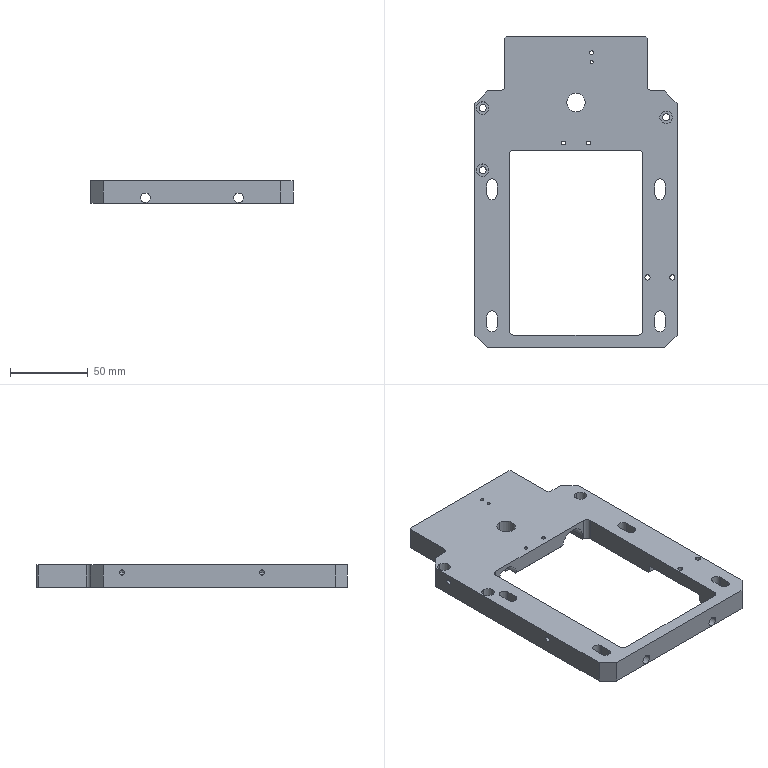NC program | NX | posted with a generic post | part box 130 x 200 x 14.5 mm
Lines 9720 to 10693 of 25347:
(ZLEVEL_PROFILE_COPY_COPY , TOOL : D4)
N19366 T17 M6
N19368 G54
N19370 G17 G0 G90 X24.194 Y-32.123 B0. C0. S5500 M3
N19372 G43 Z30. H17
N19374 Z-10.4
N19376 G94 G1 X24.463 Y-32.638 F1000.
N19378 G3 X24.8 Y-32.852 R0.4
N19380 G1 X27. Y-32.945 F1650.
N19382 X100.
N19384 X102.199 Y-32.852
N19386 Y-32.784 Z-10.45
N19388 Y-32.693 Z-10.5
N19390 X100.326 Y-32.74
N19392 X100. Y-32.792
N19394 X27.
N19396 X26.674 Y-32.74
N19398 X24.8 Y-32.693
N19400 Y-32.624 Z-10.55
N19402 Y-32.534 Z-10.6
N19404 X26.674 Y-32.58
N19406 X27. Y-32.631
N19408 X100.
N19410 X100.326 Y-32.58
N19412 X102.199 Y-32.534
N19414 Y-32.454 Z-10.65
N19416 Y-32.365 Z-10.7
N19418 X99.839 Y-32.463
N19420 X27.
N19422 X26.674 Y-32.416
N19424 X24.8 Y-32.365
N19426 Y-32.274 Z-10.75
N19428 Y-32.186 Z-10.8
N19430 X26.674 Y-32.236
N19432 X27. Y-32.286
N19434 X100.
N19436 X100.326 Y-32.236
N19438 X102.199 Y-32.186
N19440 Y-32.095 Z-10.85
N19442 Y-32.006 Z-10.9
N19444 X100.326 Y-32.056
N19446 X100. Y-32.099
N19448 X27.
N19450 X26.674 Y-32.056
N19452 X24.8 Y-32.006
N19454 Y-31.893 Z-10.95
N19456 Y-31.793 Z-11.
N19458 X27. Y-31.9
N19460 X100.
N19462 X102.199 Y-31.793
N19464 Y-31.68 Z-11.05
N19466 Y-31.567 Z-11.1
N19468 X100. Y-31.688
N19470 X27.
N19472 X24.8 Y-31.567
N19474 Y-31.453 Z-11.15
N19476 Y-31.326 Z-11.2
N19478 X26.674 Y-31.392
N19480 X27. Y-31.46
N19482 X100.
N19484 X100.326 Y-31.392
N19486 X102.199 Y-31.326
N19488 Y-31.207 Z-11.25
N19490 Y-31.071 Z-11.3
N19492 X100.326 Y-31.136
N19494 X100. Y-31.212
N19496 X27.
N19498 X26.674 Y-31.136
N19500 X24.8 Y-31.071
N19502 Y-30.937 Z-11.35
N19504 Y-30.789 Z-11.4
N19506 X26.674 Y-30.863
N19508 X27. Y-30.941
N19510 X100.
N19512 X100.326 Y-30.863
N19514 X102.199 Y-30.789
N19516 Y-30.638 Z-11.45
N19518 Y-30.49 Z-11.5
N19520 X100.326 Y-30.564
N19522 X100. Y-30.638
N19524 X27.
N19526 X26.674 Y-30.564
N19528 X24.8 Y-30.49
N19530 Y-30.304 Z-11.55
N19532 Y-30.088 Z-11.6
N19534 G2 X27. Y-30.291 R5.952
N19536 G1 X100.
N19538 G2 X102.2 Y-30.088 R6.111
N19540 G3 X102.563 Y-29.92 R0.4
N19542 G1 X104.065 Y-30.
N19544 G0 Z30.
N19546 X102.806 Y-27.877
N19548 Z-10.4
N19550 G1 X102.537 Y-27.362 F1000.
N19552 G3 X102.199 Y-27.148 R0.4
N19554 G1 X100. Y-27.055 F1650.
N19556 X27.
N19558 X24.8 Y-27.148
N19560 Y-27.216 Z-10.45
N19562 Y-27.307 Z-10.5
N19564 X26.674 Y-27.26
N19566 X27. Y-27.208
N19568 X100.
N19570 X100.326 Y-27.26
N19572 X102.199 Y-27.307
N19574 Y-27.376 Z-10.55
N19576 Y-27.466 Z-10.6
N19578 X100.326 Y-27.42
N19580 X100. Y-27.369
N19582 X27.
N19584 X26.674 Y-27.42
N19586 X24.8 Y-27.466
N19588 Y-27.546 Z-10.65
N19590 Y-27.635 Z-10.7
N19592 X26.674 Y-27.584
N19594 X27. Y-27.537
N19596 X99.839
N19598 X102.199 Y-27.635
N19600 Y-27.726 Z-10.75
N19602 Y-27.814 Z-10.8
N19604 X100.326 Y-27.764
N19606 X100. Y-27.714
N19608 X27.
N19610 X26.674 Y-27.764
N19612 X24.8 Y-27.814
N19614 Y-27.905 Z-10.85
N19616 Y-27.994 Z-10.9
N19618 X26.674 Y-27.944
N19620 X27. Y-27.901
N19622 X100.
N19624 X100.326 Y-27.944
N19626 X102.199 Y-27.994
N19628 Y-28.107 Z-10.95
N19630 Y-28.207 Z-11.
N19632 X100. Y-28.1
N19634 X27.
N19636 X24.8 Y-28.207
N19638 Y-28.32 Z-11.05
N19640 Y-28.433 Z-11.1
N19642 X27. Y-28.312
N19644 X100.
N19646 X102.199 Y-28.433
N19648 Y-28.547 Z-11.15
N19650 Y-28.674 Z-11.2
N19652 X100.326 Y-28.608
N19654 X100. Y-28.54
N19656 X27.
N19658 X26.674 Y-28.608
N19660 X24.8 Y-28.674
N19662 Y-28.793 Z-11.25
N19664 Y-28.929 Z-11.3
N19666 X26.674 Y-28.864
N19668 X27. Y-28.788
N19670 X100.
N19672 X100.326 Y-28.864
N19674 X102.199 Y-28.929
N19676 Y-29.063 Z-11.35
N19678 Y-29.211 Z-11.4
N19680 X100.326 Y-29.137
N19682 X100. Y-29.059
N19684 X27.
N19686 X26.674 Y-29.137
N19688 X24.8 Y-29.211
N19690 Y-29.362 Z-11.45
N19692 Y-29.51 Z-11.5
N19694 X26.674 Y-29.436
N19696 X27. Y-29.362
N19698 X100.
N19700 X100.326 Y-29.436
N19702 X102.199 Y-29.51
N19704 X102.2 Y-29.698 Z-11.55
N19706 Y-29.912 Z-11.6
N19708 G2 X100. Y-29.709 R5.952
N19710 G1 X27.
N19712 G2 X24.8 Y-29.912 R6.115
N19714 G3 X24.437 Y-30.08 R0.4
N19716 G1 X22.935 Y-30.
N19718 G0 Z30.
N19720 X102.825 Y32.137
N19722 Z-10.4
N19724 G1 X102.542 Y32.651 F1000.
N19726 G3 X102.199 Y32.857 R0.4
N19728 G1 X100.42 Y32.892 F1650.
N19730 X100. Y32.945
N19732 X27.
N19734 X24.8 Y32.854
N19736 Y32.785 Z-10.45
N19738 Y32.705 Z-10.5
N19740 X26.68 Y32.748
N19742 X27. Y32.792
N19744 X100.
N19746 X100.42 Y32.742
N19748 X102.199 Y32.708
N19750 Y32.623 Z-10.55
N19752 Y32.548 Z-10.6
N19754 X100. Y32.631
N19756 X27.
N19758 X24.8 Y32.545
N19760 Y32.454 Z-10.65
N19762 Y32.365 Z-10.7
N19764 X26.68 Y32.417
N19766 X27. Y32.463
N19768 X100.
N19770 X100.42 Y32.409
N19772 X102.199 Y32.369
N19774 Y32.274 Z-10.75
N19776 Y32.189 Z-10.8
N19778 X100.42 Y32.23
N19780 X100. Y32.286
N19782 X27.
N19784 X26.68 Y32.237
N19786 X24.8 Y32.186
N19788 Y32.094 Z-10.85
N19790 Y31.988 Z-10.9
N19792 X26.68 Y32.047
N19794 X27. Y32.099
N19796 X100.
N19798 X100.42 Y32.038
N19800 X102.199 Y31.992
N19802 Y31.894 Z-10.95
N19804 Y31.785 Z-11.
N19806 X100.42 Y31.83
N19808 X100. Y31.9
N19810 X27.
N19812 X26.68 Y31.838
N19814 X24.8 Y31.781
N19816 Y31.68 Z-11.05
N19818 Y31.566 Z-11.1
N19820 X26.832 Y31.642
N19822 X27. Y31.688
N19824 X100.
N19826 X100.168 Y31.642
N19828 X102.199 Y31.57
N19830 Y31.453 Z-11.15
N19832 Y31.338 Z-11.2
N19834 X101.885 Y31.334
N19836 X100. Y31.46
N19838 X27.
N19840 X26.68 Y31.395
N19842 X24.8 Y31.335
N19844 Y31.207 Z-11.25
N19846 Y31.087 Z-11.3
N19848 X26.68 Y31.161
N19850 X27. Y31.212
N19852 X100.
N19854 X101.885 Y31.086
N19856 X102.199 Y31.091
N19858 Y30.937 Z-11.35
N19860 Y30.792 Z-11.4
N19862 X100.42 Y30.852
N19864 X100. Y30.941
N19866 X27.
N19868 X26.68 Y30.864
N19870 X24.8 Y30.789
N19872 Y30.637 Z-11.45
N19874 Y30.459 Z-11.5
N19876 X26.68 Y30.545
N19878 X27. Y30.638
N19880 X100.
N19882 X100.42 Y30.531
N19884 X102.199 Y30.463
N19886 X102.201 Y30.304 Z-11.55
N19888 X102.204 Y30.092 Z-11.6
N19890 G2 X100. Y30.291 R6.23
N19892 G1 X27.
N19894 G2 X24.803 Y30.092 R6.337
N19896 G3 X24.441 Y29.921 R0.4
N19898 G1 X22.932 Y29.999
N19900 G0 Z30.
N19902 X24.191 Y27.869
N19904 Z-10.4
N19906 G1 X24.462 Y27.354 F1000.
N19908 G3 X24.8 Y27.141 R0.4
N19910 G1 X27. Y27.055 F1650.
N19912 X100.
N19914 X100.42 Y27.102
N19916 X102.199 Y27.137
N19918 Y27.215 Z-10.45
N19920 Y27.283 Z-10.5
N19922 X100.42 Y27.248
N19924 X100. Y27.208
N19926 X27.
N19928 X24.8 Y27.287
N19930 Y27.377 Z-10.55
N19932 Y27.462 Z-10.6
N19934 X27. Y27.369
N19936 X100.
N19938 X100.42 Y27.416
N19940 X102.199 Y27.458
N19942 Y27.546 Z-10.65
N19944 Y27.634 Z-10.7
N19946 X100.42 Y27.593
N19948 X100. Y27.537
N19950 X27.
N19952 X26.68 Y27.586
N19954 X24.8 Y27.638
N19956 Y27.726 Z-10.75
N19958 Y27.818 Z-10.8
N19960 X26.68 Y27.763
N19962 X27. Y27.714
N19964 X100.
N19966 X100.42 Y27.77
N19968 X102.199 Y27.814
N19970 Y27.906 Z-10.85
N19972 Y28.012 Z-10.9
N19974 X100.42 Y27.968
N19976 X100. Y27.901
N19978 X27.
N19980 X26.68 Y27.96
N19982 X24.8 Y28.015
N19984 Y28.105 Z-10.95
N19986 Y28.213 Z-11.
N19988 X26.68 Y28.159
N19990 X27. Y28.1
N19992 X100.
N19994 X100.42 Y28.167
N19996 X102.199 Y28.209
N19998 Y28.32 Z-11.05
N20000 Y28.429 Z-11.1
N20002 X101.885 Y28.433
N20004 X100. Y28.312
N20006 X27.
N20008 X24.8 Y28.432
N20010 Y28.547 Z-11.15
N20012 Y28.659 Z-11.2
N20014 X27. Y28.54
N20016 X100.
N20018 X101.885 Y28.66
N20020 X102.199 Y28.655
N20022 Y28.794 Z-11.25
N20024 Y28.92 Z-11.3
N20026 X100.42 Y28.859
N20028 X100. Y28.788
N20030 X27.
N20032 X26.68 Y28.848
N20034 X24.8 Y28.924
N20036 Y29.063 Z-11.35
N20038 Y29.212 Z-11.4
N20040 X26.68 Y29.139
N20042 X27. Y29.059
N20044 X100.
N20046 X100.42 Y29.15
N20048 X102.199 Y29.208
N20050 Y29.362 Z-11.45
N20052 Y29.532 Z-11.5
N20054 X100.42 Y29.47
N20056 X100. Y29.362
N20058 X27.
N20060 X26.68 Y29.457
N20062 X24.8 Y29.535
N20064 X24.801 Y29.696 Z-11.55
N20066 X24.803 Y29.908 Z-11.6
N20068 G2 X27. Y29.709 R6.152
N20070 G1 X100.
N20072 G2 X102.207 Y29.908 R6.355
N20074 G3 X102.569 Y30.078 R0.4
N20076 G1 X104.062 Y29.991
N20078 G0 Z30.
(ZLEVEL_PROFILE_COPY_COPY_COPY , TOOL : D4)
N20080 X-86.41 Y40.2
N20082 Z-0.1
N20084 G1 X-86.757 Y40.8 F1000.
N20086 G3 X-87.103 Y41. R0.4
N20088 G1 X-89. F1650.
N20090 G3 X-90. Y40. R1.
N20092 G1 Y38.103
N20094 G3 X-89.8 Y37.757 R0.4
N20096 G1 X-89.2 Y37.41
N20098 G0 X-86.41 Y40.2 Z-0.2
N20100 G1 X-86.757 Y40.8 F1000.
N20102 G3 X-87.103 Y41. R0.4
N20104 G1 X-89. F1650.
N20106 G3 X-90. Y40. R1.
N20108 G1 Y38.103
N20110 G3 X-89.8 Y37.757 R0.4
N20112 G1 X-89.2 Y37.41
N20114 G0 X-86.41 Y40.2 Z-0.3
N20116 G1 X-86.757 Y40.8 F1000.
N20118 G3 X-87.103 Y41. R0.4
N20120 G1 X-89. F1650.
N20122 G3 X-90. Y40. R1.
N20124 G1 Y38.103
N20126 G3 X-89.8 Y37.757 R0.4
N20128 G1 X-89.2 Y37.41
N20130 G0 X-86.41 Y40.2 Z-0.4
N20132 G1 X-86.757 Y40.8 F1000.
N20134 G3 X-87.103 Y41. R0.4
N20136 G1 X-89. F1650.
N20138 G3 X-90. Y40. R1.
N20140 G1 Y38.103
N20142 G3 X-89.8 Y37.757 R0.4
N20144 G1 X-89.2 Y37.41
N20146 G0 X-86.41 Y40.2 Z-0.5
N20148 G1 X-86.757 Y40.8 F1000.
N20150 G3 X-87.103 Y41. R0.4
N20152 G1 X-89. F1650.
N20154 G3 X-90. Y40. R1.
N20156 G1 Y38.103
N20158 G3 X-89.8 Y37.757 R0.4
N20160 G1 X-89.2 Y37.41
N20162 G0 X-86.41 Y40.2 Z-0.6
N20164 G1 X-86.757 Y40.8 F1000.
N20166 G3 X-87.103 Y41. R0.4
N20168 G1 X-89. F1650.
N20170 G3 X-90. Y40. R1.
N20172 G1 Y38.103
N20174 G3 X-89.8 Y37.757 R0.4
N20176 G1 X-89.2 Y37.41
N20178 G0 X-86.41 Y40.2 Z-0.7
N20180 G1 X-86.757 Y40.8 F1000.
N20182 G3 X-87.103 Y41. R0.4
N20184 G1 X-89. F1650.
N20186 G3 X-90. Y40. R1.
N20188 G1 Y38.103
N20190 G3 X-89.8 Y37.757 R0.4
N20192 G1 X-89.2 Y37.41
N20194 G0 X-86.41 Y40.2 Z-0.8
N20196 G1 X-86.757 Y40.8 F1000.
N20198 G3 X-87.103 Y41. R0.4
N20200 G1 X-89. F1650.
N20202 G3 X-90. Y40. R1.
N20204 G1 Y38.103
N20206 G3 X-89.8 Y37.757 R0.4
N20208 G1 X-89.2 Y37.41
N20210 G0 X-86.41 Y40.2 Z-0.9
N20212 G1 X-86.757 Y40.8 F1000.
N20214 G3 X-87.103 Y41. R0.4
N20216 G1 X-89. F1650.
N20218 G3 X-90. Y40. R1.
N20220 G1 Y38.103
N20222 G3 X-89.8 Y37.757 R0.4
N20224 G1 X-89.2 Y37.41
N20226 G0 X-86.41 Y40.2 Z-1.
N20228 G1 X-86.757 Y40.8 F1000.
N20230 G3 X-87.103 Y41. R0.4
N20232 G1 X-89. F1650.
N20234 G3 X-90. Y40. R1.
N20236 G1 Y38.103
N20238 G3 X-89.8 Y37.757 R0.4
N20240 G1 X-89.2 Y37.41
N20242 G0 X-86.41 Y40.2 Z-1.1
N20244 G1 X-86.757 Y40.8 F1000.
N20246 G3 X-87.103 Y41. R0.4
N20248 G1 X-89. F1650.
N20250 G3 X-90. Y40. R1.
N20252 G1 Y38.103
N20254 G3 X-89.8 Y37.757 R0.4
N20256 G1 X-89.2 Y37.41
N20258 G0 X-86.41 Y40.2 Z-1.2
N20260 G1 X-86.757 Y40.8 F1000.
N20262 G3 X-87.103 Y41. R0.4
N20264 G1 X-89. F1650.
N20266 G3 X-90. Y40. R1.
N20268 G1 Y38.103
N20270 G3 X-89.8 Y37.757 R0.4
N20272 G1 X-89.2 Y37.41
N20274 G0 X-86.41 Y40.2 Z-1.3
N20276 G1 X-86.757 Y40.8 F1000.
N20278 G3 X-87.103 Y41. R0.4
N20280 G1 X-89. F1650.
N20282 G3 X-90. Y40. R1.
N20284 G1 Y38.103
N20286 G3 X-89.8 Y37.757 R0.4
N20288 G1 X-89.2 Y37.41
N20290 G0 X-86.41 Y40.2 Z-1.4
N20292 G1 X-86.757 Y40.8 F1000.
N20294 G3 X-87.103 Y41. R0.4
N20296 G1 X-89. F1650.
N20298 G3 X-90. Y40. R1.
N20300 G1 Y38.103
N20302 G3 X-89.8 Y37.757 R0.4
N20304 G1 X-89.2 Y37.41
N20306 G0 X-86.41 Y40.2 Z-1.5
N20308 G1 X-86.757 Y40.8 F1000.
N20310 G3 X-87.103 Y41. R0.4
N20312 G1 X-89. F1650.
N20314 G3 X-90. Y40. R1.
N20316 G1 Y38.103
N20318 G3 X-89.8 Y37.757 R0.4
N20320 G1 X-89.2 Y37.41
N20322 G0 X-86.41 Y40.2 Z-1.6
N20324 G1 X-86.757 Y40.8 F1000.
N20326 G3 X-87.103 Y41. R0.4
N20328 G1 X-89. F1650.
N20330 G3 X-90. Y40. R1.
N20332 G1 Y38.103
N20334 G3 X-89.8 Y37.757 R0.4
N20336 G1 X-89.2 Y37.41
N20338 G0 X-86.41 Y40.2 Z-1.7
N20340 G1 X-86.757 Y40.8 F1000.
N20342 G3 X-87.103 Y41. R0.4
N20344 G1 X-89. F1650.
N20346 G3 X-90. Y40. R1.
N20348 G1 Y38.103
N20350 G3 X-89.8 Y37.757 R0.4
N20352 G1 X-89.2 Y37.41
N20354 G0 X-86.41 Y40.2 Z-1.8
N20356 G1 X-86.757 Y40.8 F1000.
N20358 G3 X-87.103 Y41. R0.4
N20360 G1 X-89. F1650.
N20362 G3 X-90. Y40. R1.
N20364 G1 Y38.103
N20366 G3 X-89.8 Y37.757 R0.4
N20368 G1 X-89.2 Y37.41
N20370 G0 X-86.41 Y40.2 Z-1.9
N20372 G1 X-86.757 Y40.8 F1000.
N20374 G3 X-87.103 Y41. R0.4
N20376 G1 X-89. F1650.
N20378 G3 X-90. Y40. R1.
N20380 G1 Y38.103
N20382 G3 X-89.8 Y37.757 R0.4
N20384 G1 X-89.2 Y37.41
N20386 G0 X-86.41 Y40.2 Z-2.
N20388 G1 X-86.757 Y40.8 F1000.
N20390 G3 X-87.103 Y41. R0.4
N20392 G1 X-89. F1650.
N20394 G3 X-90. Y40. R1.
N20396 G1 Y38.103
N20398 G3 X-89.8 Y37.757 R0.4
N20400 G1 X-89.2 Y37.41
N20402 G0 X-86.41 Y40.2 Z-2.1
N20404 G1 X-86.757 Y40.8 F1000.
N20406 G3 X-87.103 Y41. R0.4
N20408 G1 X-89. F1650.
N20410 G3 X-90. Y40. R1.
N20412 G1 Y38.103
N20414 G3 X-89.8 Y37.757 R0.4
N20416 G1 X-89.2 Y37.41
N20418 G0 X-86.41 Y40.2 Z-2.2
N20420 G1 X-86.757 Y40.8 F1000.
N20422 G3 X-87.103 Y41. R0.4
N20424 G1 X-89. F1650.
N20426 G3 X-90. Y40. R1.
N20428 G1 Y38.103
N20430 G3 X-89.8 Y37.757 R0.4
N20432 G1 X-89.2 Y37.41
N20434 G0 X-86.41 Y40.2 Z-2.3
N20436 G1 X-86.757 Y40.8 F1000.
N20438 G3 X-87.103 Y41. R0.4
N20440 G1 X-89. F1650.
N20442 G3 X-90. Y40. R1.
N20444 G1 Y38.103
N20446 G3 X-89.8 Y37.757 R0.4
N20448 G1 X-89.2 Y37.41
N20450 G0 X-86.41 Y40.2 Z-2.4
N20452 G1 X-86.757 Y40.8 F1000.
N20454 G3 X-87.103 Y41. R0.4
N20456 G1 X-89. F1650.
N20458 G3 X-90. Y40. R1.
N20460 G1 Y38.103
N20462 G3 X-89.8 Y37.757 R0.4
N20464 G1 X-89.2 Y37.41
N20466 G0 X-86.41 Y40.2 Z-2.5
N20468 G1 X-86.757 Y40.8 F1000.
N20470 G3 X-87.103 Y41. R0.4
N20472 G1 X-89. F1650.
N20474 G3 X-90. Y40. R1.
N20476 G1 Y38.103
N20478 G3 X-89.8 Y37.757 R0.4
N20480 G1 X-89.2 Y37.41
N20482 G0 X-86.41 Y40.2 Z-2.6
N20484 G1 X-86.757 Y40.8 F1000.
N20486 G3 X-87.103 Y41. R0.4
N20488 G1 X-89. F1650.
N20490 G3 X-90. Y40. R1.
N20492 G1 Y38.103
N20494 G3 X-89.8 Y37.757 R0.4
N20496 G1 X-89.2 Y37.41
N20498 G0 X-86.41 Y40.2 Z-2.7
N20500 G1 X-86.757 Y40.8 F1000.
N20502 G3 X-87.103 Y41. R0.4
N20504 G1 X-89. F1650.
N20506 G3 X-90. Y40. R1.
N20508 G1 Y38.103
N20510 G3 X-89.8 Y37.757 R0.4
N20512 G1 X-89.2 Y37.41
N20514 G0 X-86.41 Y40.2 Z-2.8
N20516 G1 X-86.757 Y40.8 F1000.
N20518 G3 X-87.103 Y41. R0.4
N20520 G1 X-89. F1650.
N20522 G3 X-90. Y40. R1.
N20524 G1 Y38.103
N20526 G3 X-89.8 Y37.757 R0.4
N20528 G1 X-89.2 Y37.41
N20530 G0 X-86.41 Y40.2 Z-2.9
N20532 G1 X-86.757 Y40.8 F1000.
N20534 G3 X-87.103 Y41. R0.4
N20536 G1 X-89. F1650.
N20538 G3 X-90. Y40. R1.
N20540 G1 Y38.103
N20542 G3 X-89.8 Y37.757 R0.4
N20544 G1 X-89.2 Y37.41
N20546 G0 X-86.41 Y40.2 Z-3.
N20548 G1 X-86.757 Y40.8 F1000.
N20550 G3 X-87.103 Y41. R0.4
N20552 G1 X-89. F1650.
N20554 G3 X-90. Y40. R1.
N20556 G1 Y38.103
N20558 G3 X-89.8 Y37.757 R0.4
N20560 G1 X-89.2 Y37.41
N20562 G0 X-86.41 Y40.2 Z-3.1
N20564 G1 X-86.757 Y40.8 F1000.
N20566 G3 X-87.103 Y41. R0.4
N20568 G1 X-89. F1650.
N20570 G3 X-90. Y40. R1.
N20572 G1 Y38.103
N20574 G3 X-89.8 Y37.757 R0.4
N20576 G1 X-89.2 Y37.41
N20578 G0 X-86.41 Y40.2 Z-3.2
N20580 G1 X-86.757 Y40.8 F1000.
N20582 G3 X-87.103 Y41. R0.4
N20584 G1 X-89. F1650.
N20586 G3 X-90. Y40. R1.
N20588 G1 Y38.103
N20590 G3 X-89.8 Y37.757 R0.4
N20592 G1 X-89.2 Y37.41
N20594 G0 X-86.41 Y40.2 Z-3.3
N20596 G1 X-86.757 Y40.8 F1000.
N20598 G3 X-87.103 Y41. R0.4
N20600 G1 X-89. F1650.
N20602 G3 X-90. Y40. R1.
N20604 G1 Y38.103
N20606 G3 X-89.8 Y37.757 R0.4
N20608 G1 X-89.2 Y37.41
N20610 G0 X-86.41 Y40.2 Z-3.4
N20612 G1 X-86.757 Y40.8 F1000.
N20614 G3 X-87.103 Y41. R0.4
N20616 G1 X-89. F1650.
N20618 G3 X-90. Y40. R1.
N20620 G1 Y38.103
N20622 G3 X-89.8 Y37.757 R0.4
N20624 G1 X-89.2 Y37.41
N20626 G0 X-86.41 Y40.2 Z-3.5
N20628 G1 X-86.757 Y40.8 F1000.
N20630 G3 X-87.103 Y41. R0.4
N20632 G1 X-89. F1650.
N20634 G3 X-90. Y40. R1.
N20636 G1 Y38.103
N20638 G3 X-89.8 Y37.757 R0.4
N20640 G1 X-89.2 Y37.41
N20642 G0 X-86.41 Y40.2 Z-3.6
N20644 G1 X-86.757 Y40.8 F1000.
N20646 G3 X-87.103 Y41. R0.4
N20648 G1 X-89. F1650.
N20650 G3 X-90. Y40. R1.
N20652 G1 Y38.103
N20654 G3 X-89.8 Y37.757 R0.4
N20656 G1 X-89.2 Y37.41
N20658 G0 X-86.41 Y40.2 Z-3.7
N20660 G1 X-86.757 Y40.8 F1000.
N20662 G3 X-87.103 Y41. R0.4
N20664 G1 X-89. F1650.
N20666 G3 X-90. Y40. R1.
N20668 G1 Y38.103
N20670 G3 X-89.8 Y37.757 R0.4
N20672 G1 X-89.2 Y37.41
N20674 G0 X-86.41 Y40.2 Z-3.8
N20676 G1 X-86.757 Y40.8 F1000.
N20678 G3 X-87.103 Y41. R0.4
N20680 G1 X-89. F1650.
N20682 G3 X-90. Y40. R1.
N20684 G1 Y38.103
N20686 G3 X-89.8 Y37.757 R0.4
N20688 G1 X-89.2 Y37.41
N20690 G0 X-86.41 Y40.2 Z-3.9
N20692 G1 X-86.757 Y40.8 F1000.
N20694 G3 X-87.103 Y41. R0.4
N20696 G1 X-89. F1650.
N20698 G3 X-90. Y40. R1.
N20700 G1 Y38.103
N20702 G3 X-89.8 Y37.757 R0.4
N20704 G1 X-89.2 Y37.41
N20706 G0 X-86.41 Y40.2 Z-4.
N20708 G1 X-86.757 Y40.8 F1000.
N20710 G3 X-87.103 Y41. R0.4
N20712 G1 X-89. F1650.
N20714 G3 X-90. Y40. R1.
N20716 G1 Y38.103
N20718 G3 X-89.8 Y37.757 R0.4
N20720 G1 X-89.2 Y37.41
N20722 G0 X-86.41 Y40.2 Z-4.1
N20724 G1 X-86.757 Y40.8 F1000.
N20726 G3 X-87.103 Y41. R0.4
N20728 G1 X-89. F1650.
N20730 G3 X-90. Y40. R1.
N20732 G1 Y38.103
N20734 G3 X-89.8 Y37.757 R0.4
N20736 G1 X-89.2 Y37.41
N20738 G0 X-86.41 Y40.2 Z-4.2
N20740 G1 X-86.757 Y40.8 F1000.
N20742 G3 X-87.103 Y41. R0.4
N20744 G1 X-89. F1650.
N20746 G3 X-90. Y40. R1.
N20748 G1 Y38.103
N20750 G3 X-89.8 Y37.757 R0.4
N20752 G1 X-89.2 Y37.41
N20754 G0 X-86.41 Y40.2 Z-4.3
N20756 G1 X-86.757 Y40.8 F1000.
N20758 G3 X-87.103 Y41. R0.4
N20760 G1 X-89. F1650.
N20762 G3 X-90. Y40. R1.
N20764 G1 Y38.103
N20766 G3 X-89.8 Y37.757 R0.4
N20768 G1 X-89.2 Y37.41
N20770 G0 X-86.41 Y40.2 Z-4.4
N20772 G1 X-86.757 Y40.8 F1000.
N20774 G3 X-87.103 Y41. R0.4
N20776 G1 X-89. F1650.
N20778 G3 X-90. Y40. R1.
N20780 G1 Y38.103
N20782 G3 X-89.8 Y37.757 R0.4
N20784 G1 X-89.2 Y37.41
N20786 G0 X-86.41 Y40.2 Z-4.5
N20788 G1 X-86.757 Y40.8 F1000.
N20790 G3 X-87.103 Y41. R0.4
N20792 G1 X-89. F1650.
N20794 G3 X-90. Y40. R1.
N20796 G1 Y38.103
N20798 G3 X-89.8 Y37.757 R0.4
N20800 G1 X-89.2 Y37.41
N20802 G0 X-86.41 Y40.2 Z-4.6
N20804 G1 X-86.757 Y40.8 F1000.
N20806 G3 X-87.103 Y41. R0.4
N20808 G1 X-89. F1650.
N20810 G3 X-90. Y40. R1.
N20812 G1 Y38.103
N20814 G3 X-89.8 Y37.757 R0.4
N20816 G1 X-89.2 Y37.41
N20818 G0 X-86.41 Y40.2 Z-4.7
N20820 G1 X-86.757 Y40.8 F1000.
N20822 G3 X-87.103 Y41. R0.4
N20824 G1 X-89. F1650.
N20826 G3 X-90. Y40. R1.
N20828 G1 Y38.103
N20830 G3 X-89.8 Y37.757 R0.4
N20832 G1 X-89.2 Y37.41
N20834 G0 X-86.41 Y40.2 Z-4.8
N20836 G1 X-86.757 Y40.8 F1000.
N20838 G3 X-87.103 Y41. R0.4
N20840 G1 X-89. F1650.
N20842 G3 X-90. Y40. R1.
N20844 G1 Y38.103
N20846 G3 X-89.8 Y37.757 R0.4
N20848 G1 X-89.2 Y37.41
N20850 G0 X-86.41 Y40.2 Z-4.9
N20852 G1 X-86.757 Y40.8 F1000.
N20854 G3 X-87.103 Y41. R0.4
N20856 G1 X-89. F1650.
N20858 G3 X-90. Y40. R1.
N20860 G1 Y38.103
N20862 G3 X-89.8 Y37.757 R0.4
N20864 G1 X-89.2 Y37.41
N20866 G0 X-86.41 Y40.2 Z-5.
N20868 G1 X-86.757 Y40.8 F1000.
N20870 G3 X-87.103 Y41. R0.4
N20872 G1 X-89. F1650.
N20874 G3 X-90. Y40. R1.
N20876 G1 Y38.103
N20878 G3 X-89.8 Y37.757 R0.4
N20880 G1 X-89.2 Y37.41
N20882 G0 X-86.41 Y40.2 Z-5.1
N20884 G1 X-86.757 Y40.8 F1000.
N20886 G3 X-87.103 Y41. R0.4
N20888 G1 X-89. F1650.
N20890 G3 X-90. Y40. R1.
N20892 G1 Y38.103
N20894 G3 X-89.8 Y37.757 R0.4
N20896 G1 X-89.2 Y37.41
N20898 G0 X-86.41 Y40.2 Z-5.2
N20900 G1 X-86.757 Y40.8 F1000.
N20902 G3 X-87.103 Y41. R0.4
N20904 G1 X-89. F1650.
N20906 G3 X-90. Y40. R1.
N20908 G1 Y38.103
N20910 G3 X-89.8 Y37.757 R0.4
N20912 G1 X-89.2 Y37.41
N20914 G0 X-86.41 Y40.2 Z-5.3
N20916 G1 X-86.757 Y40.8 F1000.
N20918 G3 X-87.103 Y41. R0.4
N20920 G1 X-89. F1650.
N20922 G3 X-90. Y40. R1.
N20924 G1 Y38.103
N20926 G3 X-89.8 Y37.757 R0.4
N20928 G1 X-89.2 Y37.41
N20930 G0 X-86.41 Y40.2 Z-5.4
N20932 G1 X-86.757 Y40.8 F1000.
N20934 G3 X-87.103 Y41. R0.4
N20936 G1 X-89. F1650.
N20938 G3 X-90. Y40. R1.
N20940 G1 Y38.103
N20942 G3 X-89.8 Y37.757 R0.4
N20944 G1 X-89.2 Y37.41
N20946 G0 X-86.41 Y40.2 Z-5.5
N20948 G1 X-86.757 Y40.8 F1000.
N20950 G3 X-87.103 Y41. R0.4
N20952 G1 X-89. F1650.
N20954 G3 X-90. Y40. R1.
N20956 G1 Y38.103
N20958 G3 X-89.8 Y37.757 R0.4
N20960 G1 X-89.2 Y37.41
N20962 G0 X-86.41 Y40.2 Z-5.6
N20964 G1 X-86.757 Y40.8 F1000.
N20966 G3 X-87.103 Y41. R0.4
N20968 G1 X-89. F1650.
N20970 G3 X-90. Y40. R1.
N20972 G1 Y38.103
N20974 G3 X-89.8 Y37.757 R0.4
N20976 G1 X-89.2 Y37.41
N20978 G0 X-86.41 Y40.2 Z-5.7
N20980 G1 X-86.757 Y40.8 F1000.
N20982 G3 X-87.103 Y41. R0.4
N20984 G1 X-89. F1650.
N20986 G3 X-90. Y40. R1.
N20988 G1 Y38.103
N20990 G3 X-89.8 Y37.757 R0.4
N20992 G1 X-89.2 Y37.41
N20994 G0 X-86.41 Y40.2 Z-5.8
N20996 G1 X-86.757 Y40.8 F1000.
N20998 G3 X-87.103 Y41. R0.4
N21000 G1 X-89. F1650.
N21002 G3 X-90. Y40. R1.
N21004 G1 Y38.103
N21006 G3 X-89.8 Y37.757 R0.4
N21008 G1 X-89.2 Y37.41
N21010 G0 X-86.41 Y40.2 Z-5.9
N21012 G1 X-86.757 Y40.8 F1000.
N21014 G3 X-87.103 Y41. R0.4
N21016 G1 X-89. F1650.
N21018 G3 X-90. Y40. R1.
N21020 G1 Y38.103
N21022 G3 X-89.8 Y37.757 R0.4
N21024 G1 X-89.2 Y37.41
N21026 G0 X-86.41 Y40.2 Z-6.
N21028 G1 X-86.757 Y40.8 F1000.
N21030 G3 X-87.103 Y41. R0.4
N21032 G1 X-89. F1650.
N21034 G3 X-90. Y40. R1.
N21036 G1 Y38.103
N21038 G3 X-89.8 Y37.757 R0.4
N21040 G1 X-89.2 Y37.41
N21042 G0 X-86.41 Y40.2 Z-6.1
N21044 G1 X-86.757 Y40.8 F1000.
N21046 G3 X-87.103 Y41. R0.4
N21048 G1 X-89. F1650.
N21050 G3 X-90. Y40. R1.
N21052 G1 Y38.103
N21054 G3 X-89.8 Y37.757 R0.4
N21056 G1 X-89.2 Y37.41
N21058 G0 X-86.41 Y40.2 Z-6.2
N21060 G1 X-86.757 Y40.8 F1000.
N21062 G3 X-87.103 Y41. R0.4
N21064 G1 X-89. F1650.
N21066 G3 X-90. Y40. R1.
N21068 G1 Y38.103
N21070 G3 X-89.8 Y37.757 R0.4
N21072 G1 X-89.2 Y37.41
N21074 G0 X-86.41 Y40.2 Z-6.3
N21076 G1 X-86.757 Y40.8 F1000.
N21078 G3 X-87.103 Y41. R0.4
N21080 G1 X-89. F1650.
N21082 G3 X-90. Y40. R1.
N21084 G1 Y38.103
N21086 G3 X-89.8 Y37.757 R0.4
N21088 G1 X-89.2 Y37.41
N21090 G0 X-86.41 Y40.2 Z-6.4
N21092 G1 X-86.757 Y40.8 F1000.
N21094 G3 X-87.103 Y41. R0.4
N21096 G1 X-89. F1650.
N21098 G3 X-90. Y40. R1.
N21100 G1 Y38.103
N21102 G3 X-89.8 Y37.757 R0.4
N21104 G1 X-89.2 Y37.41
N21106 G0 X-86.41 Y40.2 Z-6.5
N21108 G1 X-86.757 Y40.8 F1000.
N21110 G3 X-87.103 Y41. R0.4
N21112 G1 X-89. F1650.
N21114 G3 X-90. Y40. R1.
N21116 G1 Y38.103
N21118 G3 X-89.8 Y37.757 R0.4
N21120 G1 X-89.2 Y37.41
N21122 G0 X-86.41 Y40.2 Z-6.6
N21124 G1 X-86.757 Y40.8 F1000.
N21126 G3 X-87.103 Y41. R0.4
N21128 G1 X-89. F1650.
N21130 G3 X-90. Y40. R1.
N21132 G1 Y38.103
N21134 G3 X-89.8 Y37.757 R0.4
N21136 G1 X-89.2 Y37.41
N21138 G0 X-86.41 Y40.2 Z-6.7
N21140 G1 X-86.757 Y40.8 F1000.
N21142 G3 X-87.103 Y41. R0.4
N21144 G1 X-89. F1650.
N21146 G3 X-90. Y40. R1.
N21148 G1 Y38.103
N21150 G3 X-89.8 Y37.757 R0.4
N21152 G1 X-89.2 Y37.41
N21154 G0 X-86.41 Y40.2 Z-6.8
N21156 G1 X-86.757 Y40.8 F1000.
N21158 G3 X-87.103 Y41. R0.4
N21160 G1 X-89. F1650.
N21162 G3 X-90. Y40. R1.
N21164 G1 Y38.103
N21166 G3 X-89.8 Y37.757 R0.4
N21168 G1 X-89.2 Y37.41
N21170 G0 X-86.41 Y40.2 Z-6.9
N21172 G1 X-86.757 Y40.8 F1000.
N21174 G3 X-87.103 Y41. R0.4
N21176 G1 X-89. F1650.
N21178 G3 X-90. Y40. R1.
N21180 G1 Y38.103
N21182 G3 X-89.8 Y37.757 R0.4
N21184 G1 X-89.2 Y37.41
N21186 G0 X-86.41 Y40.2 Z-7.
N21188 G1 X-86.757 Y40.8 F1000.
N21190 G3 X-87.103 Y41. R0.4
N21192 G1 X-89. F1650.
N21194 G3 X-90. Y40. R1.
N21196 G1 Y38.103
N21198 G3 X-89.8 Y37.757 R0.4
N21200 G1 X-89.2 Y37.41
N21202 G0 X-86.41 Y40.2 Z-7.1
N21204 G1 X-86.757 Y40.8 F1000.
N21206 G3 X-87.103 Y41. R0.4
N21208 G1 X-89. F1650.
N21210 G3 X-90. Y40. R1.
N21212 G1 Y38.103
N21214 G3 X-89.8 Y37.757 R0.4
N21216 G1 X-89.2 Y37.41
N21218 G0 X-86.41 Y40.2 Z-7.2
N21220 G1 X-86.757 Y40.8 F1000.
N21222 G3 X-87.103 Y41. R0.4
N21224 G1 X-89. F1650.
N21226 G3 X-90. Y40. R1.
N21228 G1 Y38.103
N21230 G3 X-89.8 Y37.757 R0.4
N21232 G1 X-89.2 Y37.41
N21234 G0 X-86.41 Y40.2 Z-7.3
N21236 G1 X-86.757 Y40.8 F1000.
N21238 G3 X-87.103 Y41. R0.4
N21240 G1 X-89. F1650.
N21242 G3 X-90. Y40. R1.
N21244 G1 Y38.103
N21246 G3 X-89.8 Y37.757 R0.4
N21248 G1 X-89.2 Y37.41
N21250 G0 X-86.41 Y40.2 Z-7.4
N21252 G1 X-86.757 Y40.8 F1000.
N21254 G3 X-87.103 Y41. R0.4
N21256 G1 X-89. F1650.
N21258 G3 X-90. Y40. R1.
N21260 G1 Y38.103
N21262 G3 X-89.8 Y37.757 R0.4
N21264 G1 X-89.2 Y37.41
N21266 G0 X-86.41 Y40.2 Z-7.5
N21268 G1 X-86.757 Y40.8 F1000.
N21270 G3 X-87.103 Y41. R0.4
N21272 G1 X-89. F1650.
N21274 G3 X-90. Y40. R1.
N21276 G1 Y38.103
N21278 G3 X-89.8 Y37.757 R0.4
N21280 G1 X-89.2 Y37.41
N21282 G0 X-86.41 Y40.2 Z-7.6
N21284 G1 X-86.757 Y40.8 F1000.
N21286 G3 X-87.103 Y41. R0.4
N21288 G1 X-89. F1650.
N21290 G3 X-90. Y40. R1.
N21292 G1 Y38.103
N21294 G3 X-89.8 Y37.757 R0.4
N21296 G1 X-89.2 Y37.41
N21298 G0 X-86.41 Y40.2 Z-7.7
N21300 G1 X-86.757 Y40.8 F1000.